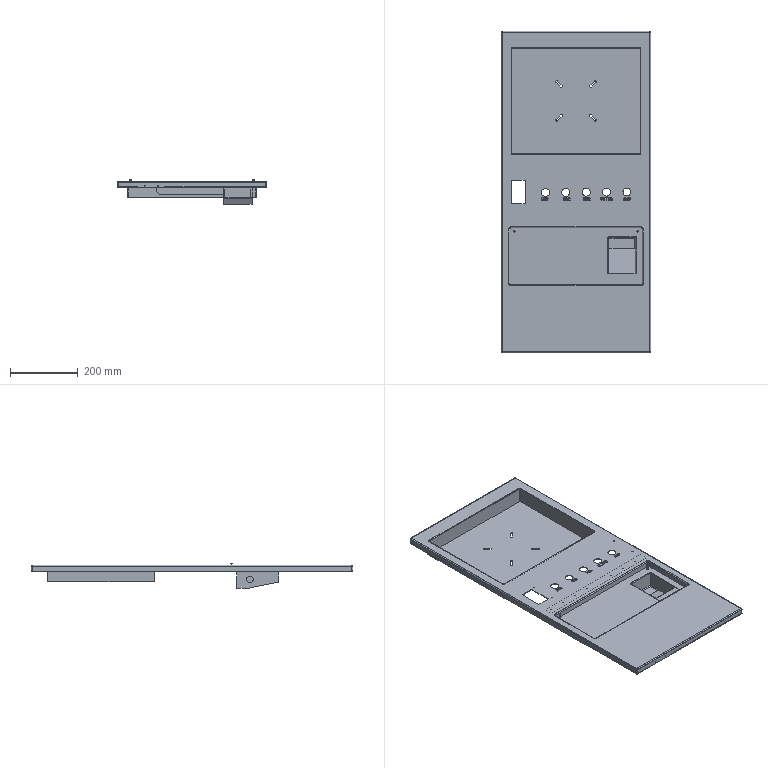Part | STEP file | 11-FG99-SHZ-010-v2.0.-V3.0-kkkkkk-998.11 | 12 solids | 732 faces | box 440 x 948 x 72 mm | volume 1225027 mm3 | plane 450 | cylinder 124 | spline 120 | cone 16 | torus 13 | sphere 9 | commonest cylinder face diameters 4 x30 2.5 x20 6 x20 2 x12 5 x12 23.5 x10